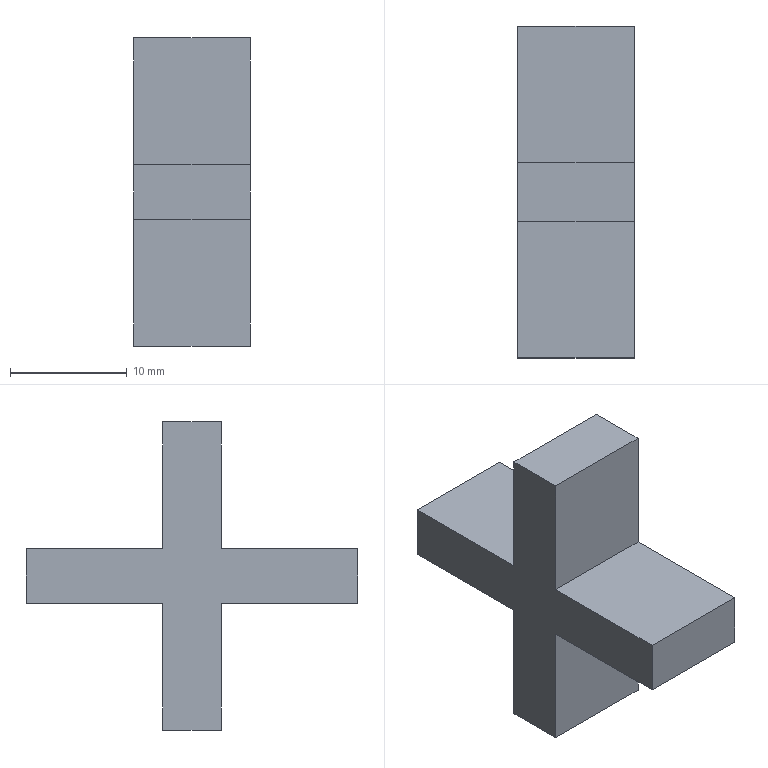Part | NX | features solid 2 | 1 solid | 14 faces | box 10 x 28.436 x 26.417 mm | volume 2421 mm3 | plane 14
STEP:
#1=CARTESIAN_POINT('',(2250.,68.934,266.792));
#2=VERTEX_POINT('',#1);
#3=CARTESIAN_POINT('',(2250.,63.902,266.792));
#4=VERTEX_POINT('',#3);
#5=CARTESIAN_POINT('',(2250.,68.934,266.792));
#6=CARTESIAN_POINT('',(2250.,67.257,266.792));
#7=CARTESIAN_POINT('',(2250.,65.579,266.792));
#8=CARTESIAN_POINT('',(2250.,63.902,266.792));
#9=B_SPLINE_CURVE_WITH_KNOTS('',3,(#5,#6,#7,#8),.UNSPECIFIED.,.F.,.F.,(4,4),(0.,0.04587),.PIECEWISE_BEZIER_KNOTS.);
#10=EDGE_CURVE('',#2,#4,#9,.T.);
#11=ORIENTED_EDGE('',*,*,#10,.F.);
#12=CARTESIAN_POINT('',(2260.,68.934,266.792));
#13=VERTEX_POINT('',#12);
#14=CARTESIAN_POINT('',(2260.,68.934,266.792));
#15=DIRECTION('',(-1.,0.,0.));
#16=VECTOR('',#15,1000.);
#17=LINE('',#14,#16);
#18=EDGE_CURVE('',#13,#2,#17,.T.);
#19=ORIENTED_EDGE('',*,*,#18,.F.);
#20=CARTESIAN_POINT('',(2260.,63.902,266.792));
#21=VERTEX_POINT('',#20);
#22=CARTESIAN_POINT('',(2260.,68.934,266.792));
#23=CARTESIAN_POINT('',(2260.,67.257,266.792));
#24=CARTESIAN_POINT('',(2260.,65.579,266.792));
#25=CARTESIAN_POINT('',(2260.,63.902,266.792));
#26=B_SPLINE_CURVE_WITH_KNOTS('',3,(#22,#23,#24,#25),.UNSPECIFIED.,.F.,.F.,(4,4),(0.,0.04587),.PIECEWISE_BEZIER_KNOTS.);
#27=EDGE_CURVE('',#13,#21,#26,.T.);
#28=ORIENTED_EDGE('',*,*,#27,.T.);
#29=CARTESIAN_POINT('',(2260.,63.902,266.792));
#30=DIRECTION('',(-1.,0.,0.));
#31=VECTOR('',#30,1000.);
#32=LINE('',#29,#31);
#33=EDGE_CURVE('',#21,#4,#32,.T.);
#34=ORIENTED_EDGE('',*,*,#33,.T.);
#35=EDGE_LOOP('',(#11,#19,#28,#34));
#36=FACE_BOUND('',#35,.T.);
#37=CARTESIAN_POINT('',(2260.,68.934,266.792));
#38=DIRECTION('',(0.,0.,-1.));
#39=DIRECTION('',(-1.,0.,0.));
#40=AXIS2_PLACEMENT_3D('',#37,#38,#39);
#41=PLANE('',#40);
#42=ADVANCED_FACE('',(#36),#41,.T.);
#43=CARTESIAN_POINT('',(2250.,63.902,277.667));
#44=VERTEX_POINT('',#43);
#45=CARTESIAN_POINT('',(2250.,63.902,266.792));
#46=CARTESIAN_POINT('',(2250.,63.902,270.417));
#47=CARTESIAN_POINT('',(2250.,63.902,274.042));
#48=CARTESIAN_POINT('',(2250.,63.902,277.667));
#49=B_SPLINE_CURVE_WITH_KNOTS('',3,(#45,#46,#47,#48),.UNSPECIFIED.,.F.,.F.,(4,4),(0.04587,0.145),.PIECEWISE_BEZIER_KNOTS.);
#50=EDGE_CURVE('',#4,#44,#49,.T.);
#51=ORIENTED_EDGE('',*,*,#50,.F.);
#52=ORIENTED_EDGE('',*,*,#33,.F.);
#53=CARTESIAN_POINT('',(2260.,63.902,277.667));
#54=VERTEX_POINT('',#53);
#55=CARTESIAN_POINT('',(2260.,63.902,266.792));
#56=CARTESIAN_POINT('',(2260.,63.902,270.417));
#57=CARTESIAN_POINT('',(2260.,63.902,274.042));
#58=CARTESIAN_POINT('',(2260.,63.902,277.667));
#59=B_SPLINE_CURVE_WITH_KNOTS('',3,(#55,#56,#57,#58),.UNSPECIFIED.,.F.,.F.,(4,4),(0.04587,0.145),.PIECEWISE_BEZIER_KNOTS.);
#60=EDGE_CURVE('',#21,#54,#59,.T.);
#61=ORIENTED_EDGE('',*,*,#60,.T.);
#62=CARTESIAN_POINT('',(2260.,63.902,277.667));
#63=DIRECTION('',(-1.,0.,0.));
#64=VECTOR('',#63,1000.);
#65=LINE('',#62,#64);
#66=EDGE_CURVE('',#54,#44,#65,.T.);
#67=ORIENTED_EDGE('',*,*,#66,.T.);
#68=EDGE_LOOP('',(#51,#52,#61,#67));
#69=FACE_BOUND('',#68,.T.);
#70=CARTESIAN_POINT('',(2260.,63.902,266.792));
#71=DIRECTION('',(0.,-1.,0.));
#72=DIRECTION('',(1.,0.,0.));
#73=AXIS2_PLACEMENT_3D('',#70,#71,#72);
#74=PLANE('',#73);
#75=ADVANCED_FACE('',(#69),#74,.T.);
#76=CARTESIAN_POINT('',(2250.,52.2,277.667));
#77=VERTEX_POINT('',#76);
#78=CARTESIAN_POINT('',(2250.,63.902,277.667));
#79=CARTESIAN_POINT('',(2250.,60.001,277.667));
#80=CARTESIAN_POINT('',(2250.,56.101,277.667));
#81=CARTESIAN_POINT('',(2250.,52.2,277.667));
#82=B_SPLINE_CURVE_WITH_KNOTS('',3,(#78,#79,#80,#81),.UNSPECIFIED.,.F.,.F.,(4,4),(0.145,0.2517),.PIECEWISE_BEZIER_KNOTS.);
#83=EDGE_CURVE('',#44,#77,#82,.T.);
#84=ORIENTED_EDGE('',*,*,#83,.F.);
#85=ORIENTED_EDGE('',*,*,#66,.F.);
#86=CARTESIAN_POINT('',(2260.,52.2,277.667));
#87=VERTEX_POINT('',#86);
#88=CARTESIAN_POINT('',(2260.,63.902,277.667));
#89=CARTESIAN_POINT('',(2260.,60.001,277.667));
#90=CARTESIAN_POINT('',(2260.,56.101,277.667));
#91=CARTESIAN_POINT('',(2260.,52.2,277.667));
#92=B_SPLINE_CURVE_WITH_KNOTS('',3,(#88,#89,#90,#91),.UNSPECIFIED.,.F.,.F.,(4,4),(0.145,0.2517),.PIECEWISE_BEZIER_KNOTS.);
#93=EDGE_CURVE('',#54,#87,#92,.T.);
#94=ORIENTED_EDGE('',*,*,#93,.T.);
#95=CARTESIAN_POINT('',(2260.,52.2,277.667));
#96=DIRECTION('',(-1.,0.,0.));
#97=VECTOR('',#96,1000.);
#98=LINE('',#95,#97);
#99=EDGE_CURVE('',#87,#77,#98,.T.);
#100=ORIENTED_EDGE('',*,*,#99,.T.);
#101=EDGE_LOOP('',(#84,#85,#94,#100));
#102=FACE_BOUND('',#101,.T.);
#103=CARTESIAN_POINT('',(2260.,63.902,277.667));
#104=DIRECTION('',(0.,0.,-1.));
#105=DIRECTION('',(-1.,0.,0.));
#106=AXIS2_PLACEMENT_3D('',#103,#104,#105);
#107=PLANE('',#106);
#108=ADVANCED_FACE('',(#102),#107,.T.);
#109=CARTESIAN_POINT('',(2250.,52.2,282.333));
#110=VERTEX_POINT('',#109);
#111=CARTESIAN_POINT('',(2250.,52.2,277.667));
#112=CARTESIAN_POINT('',(2250.,52.2,279.222));
#113=CARTESIAN_POINT('',(2250.,52.2,280.778));
#114=CARTESIAN_POINT('',(2250.,52.2,282.333));
#115=B_SPLINE_CURVE_WITH_KNOTS('',3,(#111,#112,#113,#114),.UNSPECIFIED.,.F.,.F.,(4,4),(0.2517,0.2942),.PIECEWISE_BEZIER_KNOTS.);
#116=EDGE_CURVE('',#77,#110,#115,.T.);
#117=ORIENTED_EDGE('',*,*,#116,.F.);
#118=ORIENTED_EDGE('',*,*,#99,.F.);
#119=CARTESIAN_POINT('',(2260.,52.2,282.333));
#120=VERTEX_POINT('',#119);
#121=CARTESIAN_POINT('',(2260.,52.2,277.667));
#122=CARTESIAN_POINT('',(2260.,52.2,279.222));
#123=CARTESIAN_POINT('',(2260.,52.2,280.778));
#124=CARTESIAN_POINT('',(2260.,52.2,282.333));
#125=B_SPLINE_CURVE_WITH_KNOTS('',3,(#121,#122,#123,#124),.UNSPECIFIED.,.F.,.F.,(4,4),(0.2517,0.2942),.PIECEWISE_BEZIER_KNOTS.);
#126=EDGE_CURVE('',#87,#120,#125,.T.);
#127=ORIENTED_EDGE('',*,*,#126,.T.);
#128=CARTESIAN_POINT('',(2260.,52.2,282.333));
#129=DIRECTION('',(-1.,0.,0.));
#130=VECTOR('',#129,1000.);
#131=LINE('',#128,#130);
#132=EDGE_CURVE('',#120,#110,#131,.T.);
#133=ORIENTED_EDGE('',*,*,#132,.T.);
#134=EDGE_LOOP('',(#117,#118,#127,#133));
#135=FACE_BOUND('',#134,.T.);
#136=CARTESIAN_POINT('',(2260.,52.2,277.667));
#137=DIRECTION('',(0.,-1.,0.));
#138=DIRECTION('',(1.,0.,0.));
#139=AXIS2_PLACEMENT_3D('',#136,#137,#138);
#140=PLANE('',#139);
#141=ADVANCED_FACE('',(#135),#140,.T.);
#142=CARTESIAN_POINT('',(2250.,63.902,282.333));
#143=VERTEX_POINT('',#142);
#144=CARTESIAN_POINT('',(2250.,52.2,282.333));
#145=CARTESIAN_POINT('',(2250.,56.101,282.333));
#146=CARTESIAN_POINT('',(2250.,60.001,282.333));
#147=CARTESIAN_POINT('',(2250.,63.902,282.333));
#148=B_SPLINE_CURVE_WITH_KNOTS('',3,(#144,#145,#146,#147),.UNSPECIFIED.,.F.,.F.,(4,4),(0.2942,0.4009),.PIECEWISE_BEZIER_KNOTS.);
#149=EDGE_CURVE('',#110,#143,#148,.T.);
#150=ORIENTED_EDGE('',*,*,#149,.F.);
#151=ORIENTED_EDGE('',*,*,#132,.F.);
#152=CARTESIAN_POINT('',(2260.,63.902,282.333));
#153=VERTEX_POINT('',#152);
#154=CARTESIAN_POINT('',(2260.,52.2,282.333));
#155=CARTESIAN_POINT('',(2260.,56.101,282.333));
#156=CARTESIAN_POINT('',(2260.,60.001,282.333));
#157=CARTESIAN_POINT('',(2260.,63.902,282.333));
#158=B_SPLINE_CURVE_WITH_KNOTS('',3,(#154,#155,#156,#157),.UNSPECIFIED.,.F.,.F.,(4,4),(0.2942,0.4009),.PIECEWISE_BEZIER_KNOTS.);
#159=EDGE_CURVE('',#120,#153,#158,.T.);
#160=ORIENTED_EDGE('',*,*,#159,.T.);
#161=CARTESIAN_POINT('',(2260.,63.902,282.333));
#162=DIRECTION('',(-1.,0.,0.));
#163=VECTOR('',#162,1000.);
#164=LINE('',#161,#163);
#165=EDGE_CURVE('',#153,#143,#164,.T.);
#166=ORIENTED_EDGE('',*,*,#165,.T.);
#167=EDGE_LOOP('',(#150,#151,#160,#166));
#168=FACE_BOUND('',#167,.T.);
#169=CARTESIAN_POINT('',(2260.,52.2,282.333));
#170=DIRECTION('',(0.,0.,1.));
#171=DIRECTION('',(1.,0.,0.));
#172=AXIS2_PLACEMENT_3D('',#169,#170,#171);
#173=PLANE('',#172);
#174=ADVANCED_FACE('',(#168),#173,.T.);
#175=CARTESIAN_POINT('',(2250.,63.902,293.208));
#176=VERTEX_POINT('',#175);
#177=CARTESIAN_POINT('',(2250.,63.902,282.333));
#178=CARTESIAN_POINT('',(2250.,63.902,285.958));
#179=CARTESIAN_POINT('',(2250.,63.902,289.583));
#180=CARTESIAN_POINT('',(2250.,63.902,293.208));
#181=B_SPLINE_CURVE_WITH_KNOTS('',3,(#177,#178,#179,#180),.UNSPECIFIED.,.F.,.F.,(4,4),(0.4009,0.5),.PIECEWISE_BEZIER_KNOTS.);
#182=EDGE_CURVE('',#143,#176,#181,.T.);
#183=ORIENTED_EDGE('',*,*,#182,.F.);
#184=ORIENTED_EDGE('',*,*,#165,.F.);
#185=CARTESIAN_POINT('',(2260.,63.902,293.208));
#186=VERTEX_POINT('',#185);
#187=CARTESIAN_POINT('',(2260.,63.902,282.333));
#188=CARTESIAN_POINT('',(2260.,63.902,285.958));
#189=CARTESIAN_POINT('',(2260.,63.902,289.583));
#190=CARTESIAN_POINT('',(2260.,63.902,293.208));
#191=B_SPLINE_CURVE_WITH_KNOTS('',3,(#187,#188,#189,#190),.UNSPECIFIED.,.F.,.F.,(4,4),(0.4009,0.5),.PIECEWISE_BEZIER_KNOTS.);
#192=EDGE_CURVE('',#153,#186,#191,.T.);
#193=ORIENTED_EDGE('',*,*,#192,.T.);
#194=CARTESIAN_POINT('',(2260.,63.902,293.208));
#195=DIRECTION('',(-1.,0.,0.));
#196=VECTOR('',#195,1000.);
#197=LINE('',#194,#196);
#198=EDGE_CURVE('',#186,#176,#197,.T.);
#199=ORIENTED_EDGE('',*,*,#198,.T.);
#200=EDGE_LOOP('',(#183,#184,#193,#199));
#201=FACE_BOUND('',#200,.T.);
#202=CARTESIAN_POINT('',(2260.,63.902,282.333));
#203=DIRECTION('',(0.,-1.,0.));
#204=DIRECTION('',(1.,0.,0.));
#205=AXIS2_PLACEMENT_3D('',#202,#203,#204);
#206=PLANE('',#205);
#207=ADVANCED_FACE('',(#201),#206,.T.);
#208=CARTESIAN_POINT('',(2250.,68.934,293.208));
#209=VERTEX_POINT('',#208);
#210=CARTESIAN_POINT('',(2250.,63.902,293.208));
#211=CARTESIAN_POINT('',(2250.,65.579,293.208));
#212=CARTESIAN_POINT('',(2250.,67.257,293.208));
#213=CARTESIAN_POINT('',(2250.,68.934,293.208));
#214=B_SPLINE_CURVE_WITH_KNOTS('',3,(#210,#211,#212,#213),.UNSPECIFIED.,.F.,.F.,(4,4),(0.5,0.5459),.PIECEWISE_BEZIER_KNOTS.);
#215=EDGE_CURVE('',#176,#209,#214,.T.);
#216=ORIENTED_EDGE('',*,*,#215,.F.);
#217=ORIENTED_EDGE('',*,*,#198,.F.);
#218=CARTESIAN_POINT('',(2260.,68.934,293.208));
#219=VERTEX_POINT('',#218);
#220=CARTESIAN_POINT('',(2260.,63.902,293.208));
#221=CARTESIAN_POINT('',(2260.,65.579,293.208));
#222=CARTESIAN_POINT('',(2260.,67.257,293.208));
#223=CARTESIAN_POINT('',(2260.,68.934,293.208));
#224=B_SPLINE_CURVE_WITH_KNOTS('',3,(#220,#221,#222,#223),.UNSPECIFIED.,.F.,.F.,(4,4),(0.5,0.5459),.PIECEWISE_BEZIER_KNOTS.);
#225=EDGE_CURVE('',#186,#219,#224,.T.);
#226=ORIENTED_EDGE('',*,*,#225,.T.);
#227=CARTESIAN_POINT('',(2260.,68.934,293.208));
#228=DIRECTION('',(-1.,0.,0.));
#229=VECTOR('',#228,1000.);
#230=LINE('',#227,#229);
#231=EDGE_CURVE('',#219,#209,#230,.T.);
#232=ORIENTED_EDGE('',*,*,#231,.T.);
#233=EDGE_LOOP('',(#216,#217,#226,#232));
#234=FACE_BOUND('',#233,.T.);
#235=CARTESIAN_POINT('',(2260.,63.902,293.208));
#236=DIRECTION('',(0.,0.,1.));
#237=DIRECTION('',(1.,0.,0.));
#238=AXIS2_PLACEMENT_3D('',#235,#236,#237);
#239=PLANE('',#238);
#240=ADVANCED_FACE('',(#234),#239,.T.);
#241=CARTESIAN_POINT('',(2250.,68.934,282.333));
#242=VERTEX_POINT('',#241);
#243=CARTESIAN_POINT('',(2250.,68.934,293.208));
#244=CARTESIAN_POINT('',(2250.,68.934,289.583));
#245=CARTESIAN_POINT('',(2250.,68.934,285.958));
#246=CARTESIAN_POINT('',(2250.,68.934,282.333));
#247=B_SPLINE_CURVE_WITH_KNOTS('',3,(#243,#244,#245,#246),.UNSPECIFIED.,.F.,.F.,(4,4),(0.5459,0.645),.PIECEWISE_BEZIER_KNOTS.);
#248=EDGE_CURVE('',#209,#242,#247,.T.);
#249=ORIENTED_EDGE('',*,*,#248,.F.);
#250=ORIENTED_EDGE('',*,*,#231,.F.);
#251=CARTESIAN_POINT('',(2260.,68.934,282.333));
#252=VERTEX_POINT('',#251);
#253=CARTESIAN_POINT('',(2260.,68.934,293.208));
#254=CARTESIAN_POINT('',(2260.,68.934,289.583));
#255=CARTESIAN_POINT('',(2260.,68.934,285.958));
#256=CARTESIAN_POINT('',(2260.,68.934,282.333));
#257=B_SPLINE_CURVE_WITH_KNOTS('',3,(#253,#254,#255,#256),.UNSPECIFIED.,.F.,.F.,(4,4),(0.5459,0.645),.PIECEWISE_BEZIER_KNOTS.);
#258=EDGE_CURVE('',#219,#252,#257,.T.);
#259=ORIENTED_EDGE('',*,*,#258,.T.);
#260=CARTESIAN_POINT('',(2260.,68.934,282.333));
#261=DIRECTION('',(-1.,0.,0.));
#262=VECTOR('',#261,1000.);
#263=LINE('',#260,#262);
#264=EDGE_CURVE('',#252,#242,#263,.T.);
#265=ORIENTED_EDGE('',*,*,#264,.T.);
#266=EDGE_LOOP('',(#249,#250,#259,#265));
#267=FACE_BOUND('',#266,.T.);
#268=CARTESIAN_POINT('',(2260.,68.934,293.208));
#269=DIRECTION('',(0.,1.,0.));
#270=DIRECTION('',(-1.,0.,0.));
#271=AXIS2_PLACEMENT_3D('',#268,#269,#270);
#272=PLANE('',#271);
#273=ADVANCED_FACE('',(#267),#272,.T.);
#274=CARTESIAN_POINT('',(2250.,80.636,282.333));
#275=VERTEX_POINT('',#274);
#276=CARTESIAN_POINT('',(2250.,68.934,282.333));
#277=CARTESIAN_POINT('',(2250.,72.835,282.333));
#278=CARTESIAN_POINT('',(2250.,76.735,282.333));
#279=CARTESIAN_POINT('',(2250.,80.636,282.333));
#280=B_SPLINE_CURVE_WITH_KNOTS('',3,(#276,#277,#278,#279),.UNSPECIFIED.,.F.,.F.,(4,4),(0.645,0.7517),.PIECEWISE_BEZIER_KNOTS.);
#281=EDGE_CURVE('',#242,#275,#280,.T.);
#282=ORIENTED_EDGE('',*,*,#281,.F.);
#283=ORIENTED_EDGE('',*,*,#264,.F.);
#284=CARTESIAN_POINT('',(2260.,80.636,282.333));
#285=VERTEX_POINT('',#284);
#286=CARTESIAN_POINT('',(2260.,68.934,282.333));
#287=CARTESIAN_POINT('',(2260.,72.835,282.333));
#288=CARTESIAN_POINT('',(2260.,76.735,282.333));
#289=CARTESIAN_POINT('',(2260.,80.636,282.333));
#290=B_SPLINE_CURVE_WITH_KNOTS('',3,(#286,#287,#288,#289),.UNSPECIFIED.,.F.,.F.,(4,4),(0.645,0.7517),.PIECEWISE_BEZIER_KNOTS.);
#291=EDGE_CURVE('',#252,#285,#290,.T.);
#292=ORIENTED_EDGE('',*,*,#291,.T.);
#293=CARTESIAN_POINT('',(2260.,80.636,282.333));
#294=DIRECTION('',(-1.,0.,0.));
#295=VECTOR('',#294,1000.);
#296=LINE('',#293,#295);
#297=EDGE_CURVE('',#285,#275,#296,.T.);
#298=ORIENTED_EDGE('',*,*,#297,.T.);
#299=EDGE_LOOP('',(#282,#283,#292,#298));
#300=FACE_BOUND('',#299,.T.);
#301=CARTESIAN_POINT('',(2260.,68.934,282.333));
#302=DIRECTION('',(0.,0.,1.));
#303=DIRECTION('',(1.,0.,0.));
#304=AXIS2_PLACEMENT_3D('',#301,#302,#303);
#305=PLANE('',#304);
#306=ADVANCED_FACE('',(#300),#305,.T.);
#307=CARTESIAN_POINT('',(2250.,80.636,277.667));
#308=VERTEX_POINT('',#307);
#309=CARTESIAN_POINT('',(2250.,80.636,282.333));
#310=CARTESIAN_POINT('',(2250.,80.636,280.778));
#311=CARTESIAN_POINT('',(2250.,80.636,279.222));
#312=CARTESIAN_POINT('',(2250.,80.636,277.667));
#313=B_SPLINE_CURVE_WITH_KNOTS('',3,(#309,#310,#311,#312),.UNSPECIFIED.,.F.,.F.,(4,4),(0.7517,0.7942),.PIECEWISE_BEZIER_KNOTS.);
#314=EDGE_CURVE('',#275,#308,#313,.T.);
#315=ORIENTED_EDGE('',*,*,#314,.F.);
#316=ORIENTED_EDGE('',*,*,#297,.F.);
#317=CARTESIAN_POINT('',(2260.,80.636,277.667));
#318=VERTEX_POINT('',#317);
#319=CARTESIAN_POINT('',(2260.,80.636,282.333));
#320=CARTESIAN_POINT('',(2260.,80.636,280.778));
#321=CARTESIAN_POINT('',(2260.,80.636,279.222));
#322=CARTESIAN_POINT('',(2260.,80.636,277.667));
#323=B_SPLINE_CURVE_WITH_KNOTS('',3,(#319,#320,#321,#322),.UNSPECIFIED.,.F.,.F.,(4,4),(0.7517,0.7942),.PIECEWISE_BEZIER_KNOTS.);
#324=EDGE_CURVE('',#285,#318,#323,.T.);
#325=ORIENTED_EDGE('',*,*,#324,.T.);
#326=CARTESIAN_POINT('',(2260.,80.636,277.667));
#327=DIRECTION('',(-1.,0.,0.));
#328=VECTOR('',#327,1000.);
#329=LINE('',#326,#328);
#330=EDGE_CURVE('',#318,#308,#329,.T.);
#331=ORIENTED_EDGE('',*,*,#330,.T.);
#332=EDGE_LOOP('',(#315,#316,#325,#331));
#333=FACE_BOUND('',#332,.T.);
#334=CARTESIAN_POINT('',(2260.,80.636,282.333));
#335=DIRECTION('',(0.,1.,0.));
#336=DIRECTION('',(-1.,0.,0.));
#337=AXIS2_PLACEMENT_3D('',#334,#335,#336);
#338=PLANE('',#337);
#339=ADVANCED_FACE('',(#333),#338,.T.);
#340=CARTESIAN_POINT('',(2250.,68.934,277.667));
#341=VERTEX_POINT('',#340);
#342=CARTESIAN_POINT('',(2250.,80.636,277.667));
#343=CARTESIAN_POINT('',(2250.,76.735,277.667));
#344=CARTESIAN_POINT('',(2250.,72.835,277.667));
#345=CARTESIAN_POINT('',(2250.,68.934,277.667));
#346=B_SPLINE_CURVE_WITH_KNOTS('',3,(#342,#343,#344,#345),.UNSPECIFIED.,.F.,.F.,(4,4),(0.7942,0.9009),.PIECEWISE_BEZIER_KNOTS.);
#347=EDGE_CURVE('',#308,#341,#346,.T.);
#348=ORIENTED_EDGE('',*,*,#347,.F.);
#349=ORIENTED_EDGE('',*,*,#330,.F.);
#350=CARTESIAN_POINT('',(2260.,68.934,277.667));
#351=VERTEX_POINT('',#350);
#352=CARTESIAN_POINT('',(2260.,80.636,277.667));
#353=CARTESIAN_POINT('',(2260.,76.735,277.667));
#354=CARTESIAN_POINT('',(2260.,72.835,277.667));
#355=CARTESIAN_POINT('',(2260.,68.934,277.667));
#356=B_SPLINE_CURVE_WITH_KNOTS('',3,(#352,#353,#354,#355),.UNSPECIFIED.,.F.,.F.,(4,4),(0.7942,0.9009),.PIECEWISE_BEZIER_KNOTS.);
#357=EDGE_CURVE('',#318,#351,#356,.T.);
#358=ORIENTED_EDGE('',*,*,#357,.T.);
#359=CARTESIAN_POINT('',(2260.,68.934,277.667));
#360=DIRECTION('',(-1.,0.,0.));
#361=VECTOR('',#360,1000.);
#362=LINE('',#359,#361);
#363=EDGE_CURVE('',#351,#341,#362,.T.);
#364=ORIENTED_EDGE('',*,*,#363,.T.);
#365=EDGE_LOOP('',(#348,#349,#358,#364));
#366=FACE_BOUND('',#365,.T.);
#367=CARTESIAN_POINT('',(2260.,80.636,277.667));
#368=DIRECTION('',(0.,0.,-1.));
#369=DIRECTION('',(-1.,0.,0.));
#370=AXIS2_PLACEMENT_3D('',#367,#368,#369);
#371=PLANE('',#370);
#372=ADVANCED_FACE('',(#366),#371,.T.);
#373=CARTESIAN_POINT('',(2250.,68.934,277.667));
#374=CARTESIAN_POINT('',(2250.,68.934,274.042));
#375=CARTESIAN_POINT('',(2250.,68.934,270.417));
#376=CARTESIAN_POINT('',(2250.,68.934,266.792));
#377=B_SPLINE_CURVE_WITH_KNOTS('',3,(#373,#374,#375,#376),.UNSPECIFIED.,.F.,.F.,(4,4),(0.9009,1.),.PIECEWISE_BEZIER_KNOTS.);
#378=EDGE_CURVE('',#341,#2,#377,.T.);
#379=ORIENTED_EDGE('',*,*,#378,.F.);
#380=ORIENTED_EDGE('',*,*,#363,.F.);
#381=CARTESIAN_POINT('',(2260.,68.934,277.667));
#382=CARTESIAN_POINT('',(2260.,68.934,274.042));
#383=CARTESIAN_POINT('',(2260.,68.934,270.417));
#384=CARTESIAN_POINT('',(2260.,68.934,266.792));
#385=B_SPLINE_CURVE_WITH_KNOTS('',3,(#381,#382,#383,#384),.UNSPECIFIED.,.F.,.F.,(4,4),(0.9009,1.),.PIECEWISE_BEZIER_KNOTS.);
#386=EDGE_CURVE('',#351,#13,#385,.T.);
#387=ORIENTED_EDGE('',*,*,#386,.T.);
#388=ORIENTED_EDGE('',*,*,#18,.T.);
#389=EDGE_LOOP('',(#379,#380,#387,#388));
#390=FACE_BOUND('',#389,.T.);
#391=CARTESIAN_POINT('',(2260.,68.934,277.667));
#392=DIRECTION('',(0.,1.,0.));
#393=DIRECTION('',(-1.,0.,0.));
#394=AXIS2_PLACEMENT_3D('',#391,#392,#393);
#395=PLANE('',#394);
#396=ADVANCED_FACE('',(#390),#395,.T.);
#397=ORIENTED_EDGE('',*,*,#27,.F.);
#398=ORIENTED_EDGE('',*,*,#386,.F.);
#399=ORIENTED_EDGE('',*,*,#357,.F.);
#400=ORIENTED_EDGE('',*,*,#324,.F.);
#401=ORIENTED_EDGE('',*,*,#291,.F.);
#402=ORIENTED_EDGE('',*,*,#258,.F.);
#403=ORIENTED_EDGE('',*,*,#225,.F.);
#404=ORIENTED_EDGE('',*,*,#192,.F.);
#405=ORIENTED_EDGE('',*,*,#159,.F.);
#406=ORIENTED_EDGE('',*,*,#126,.F.);
#407=ORIENTED_EDGE('',*,*,#93,.F.);
#408=ORIENTED_EDGE('',*,*,#60,.F.);
#409=EDGE_LOOP('',(#397,#398,#399,#400,#401,#402,#403,#404,#405,#406,#407,#408));
#410=FACE_BOUND('',#409,.T.);
#411=CARTESIAN_POINT('',(2260.,66.418,266.792));
#412=DIRECTION('',(1.,0.,0.));
#413=DIRECTION('',(0.,1.,0.));
#414=AXIS2_PLACEMENT_3D('',#411,#412,#413);
#415=PLANE('',#414);
#416=ADVANCED_FACE('',(#410),#415,.T.);
#417=ORIENTED_EDGE('',*,*,#10,.T.);
#418=ORIENTED_EDGE('',*,*,#50,.T.);
#419=ORIENTED_EDGE('',*,*,#83,.T.);
#420=ORIENTED_EDGE('',*,*,#116,.T.);
#421=ORIENTED_EDGE('',*,*,#149,.T.);
#422=ORIENTED_EDGE('',*,*,#182,.T.);
#423=ORIENTED_EDGE('',*,*,#215,.T.);
#424=ORIENTED_EDGE('',*,*,#248,.T.);
#425=ORIENTED_EDGE('',*,*,#281,.T.);
#426=ORIENTED_EDGE('',*,*,#314,.T.);
#427=ORIENTED_EDGE('',*,*,#347,.T.);
#428=ORIENTED_EDGE('',*,*,#378,.T.);
#429=EDGE_LOOP('',(#417,#418,#419,#420,#421,#422,#423,#424,#425,#426,#427,#428));
#430=FACE_BOUND('',#429,.T.);
#431=CARTESIAN_POINT('',(2250.,66.418,266.792));
#432=DIRECTION('',(1.,0.,0.));
#433=DIRECTION('',(0.,1.,0.));
#434=AXIS2_PLACEMENT_3D('',#431,#432,#433);
#435=PLANE('',#434);
#436=ADVANCED_FACE('',(#430),#435,.F.);
#437=CLOSED_SHELL('',(#42,#75,#108,#141,#174,#207,#240,#273,#306,#339,#372,#396,#416,#436));
#438=MANIFOLD_SOLID_BREP('',#437);
#439=(LENGTH_UNIT()NAMED_UNIT(*)SI_UNIT(.MILLI.,.METRE.));
#440=UNCERTAINTY_MEASURE_WITH_UNIT(LENGTH_MEASURE(0.00001),#439,'','');
#441=(NAMED_UNIT(*)PLANE_ANGLE_UNIT()SI_UNIT($,.RADIAN.));
#442=(NAMED_UNIT(*)SI_UNIT($,.STERADIAN.)SOLID_ANGLE_UNIT());
#443=(GEOMETRIC_REPRESENTATION_CONTEXT(3)GLOBAL_UNCERTAINTY_ASSIGNED_CONTEXT((#440))GLOBAL_UNIT_ASSIGNED_CONTEXT((#439,#441,#442))REPRESENTATION_CONTEXT('',''));
#444=ADVANCED_BREP_SHAPE_REPRESENTATION('',(#438),#443);